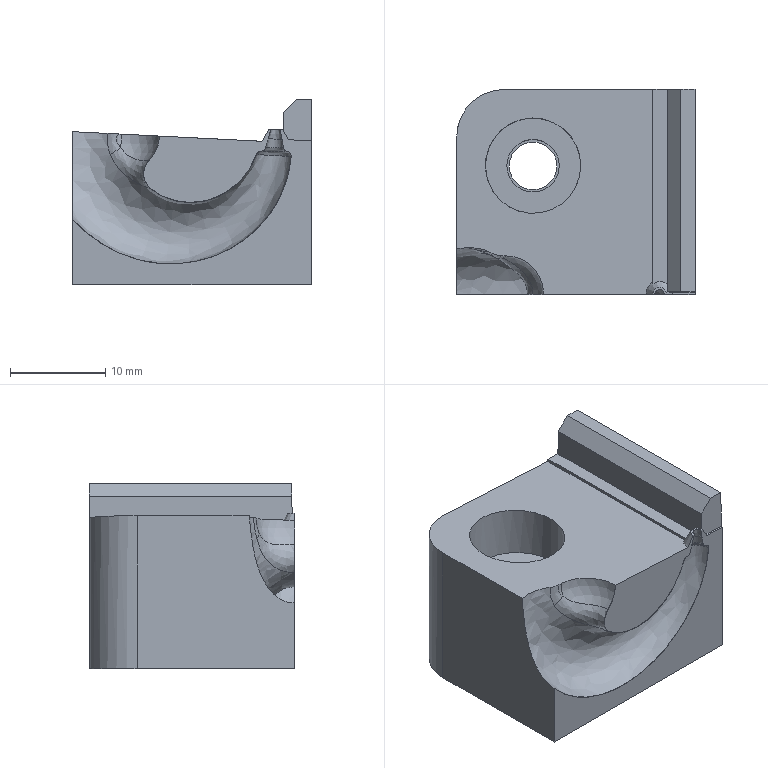Part | STEP file | solid 194 | 1 solid | 39 faces | box 25 x 21.5 x 19.435 mm | volume 7259 mm3 | plane 15 | spline 15 | cylinder 6 | sphere 2 | cone 1 | commonest cylinder face diameters 10 x2 5 x1 5.5 x1 8 x1 6922 x1